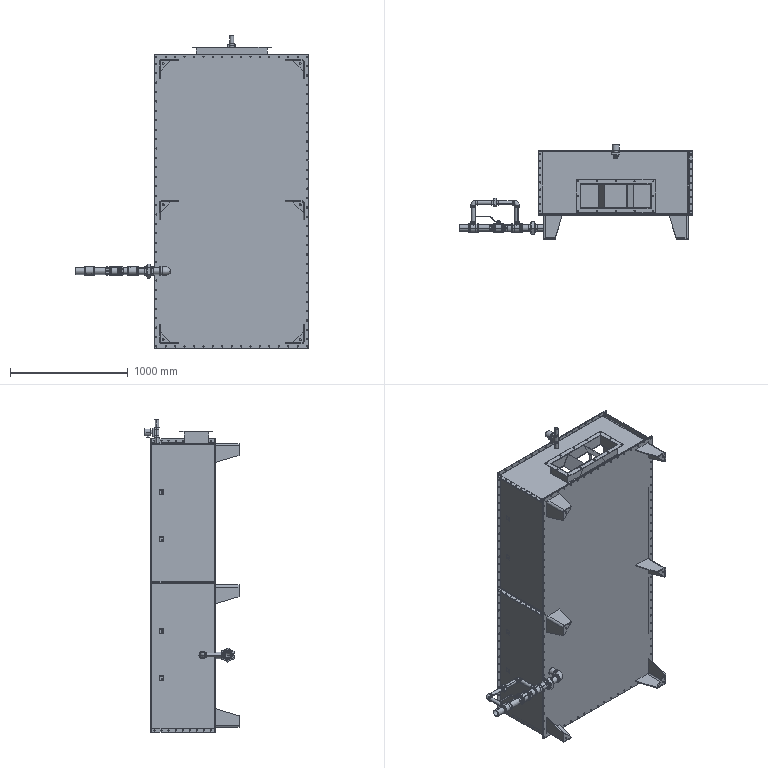Part | SolidWorks | features ReferencePattern 3, LocalLPattern 2 | 205 solids | 4355 faces | volume 52645263 mm3 | cylinder 1929 | plane 1875 | cone 444 | torus 107 | commonest cylinder face diameters 10 x916 20 x213 25 x93 16 x84 4 x48 4.1 x36